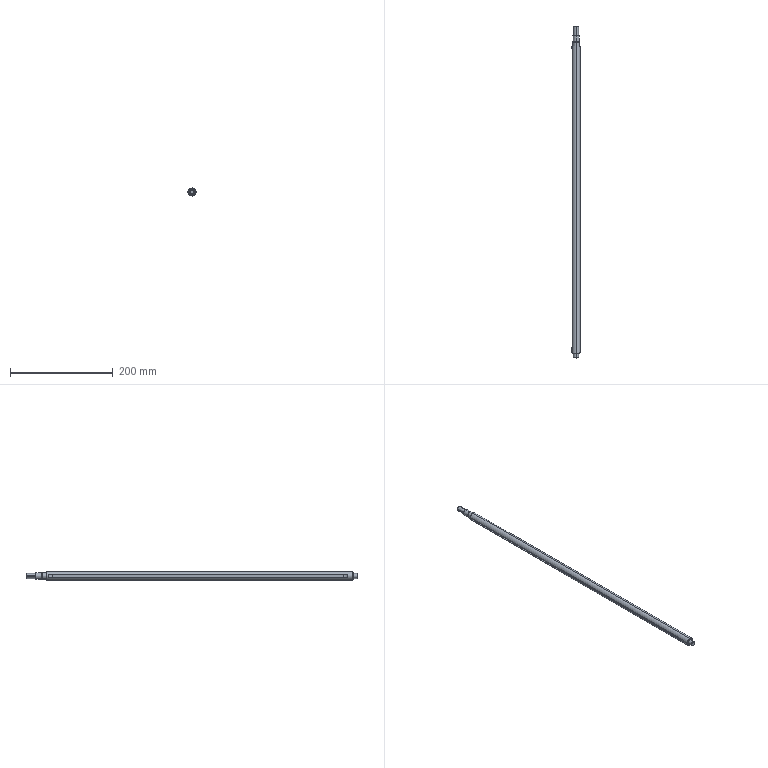Part | STEP file | 1 solid | 37 faces | box 16 x 647 x 16 mm | volume 120315 mm3 | cylinder 14 | plane 13 | cone 8 | spline 2 | commonest cylinder face diameters 10 x4 12 x4 3 x2 11.2 x2 16 x2